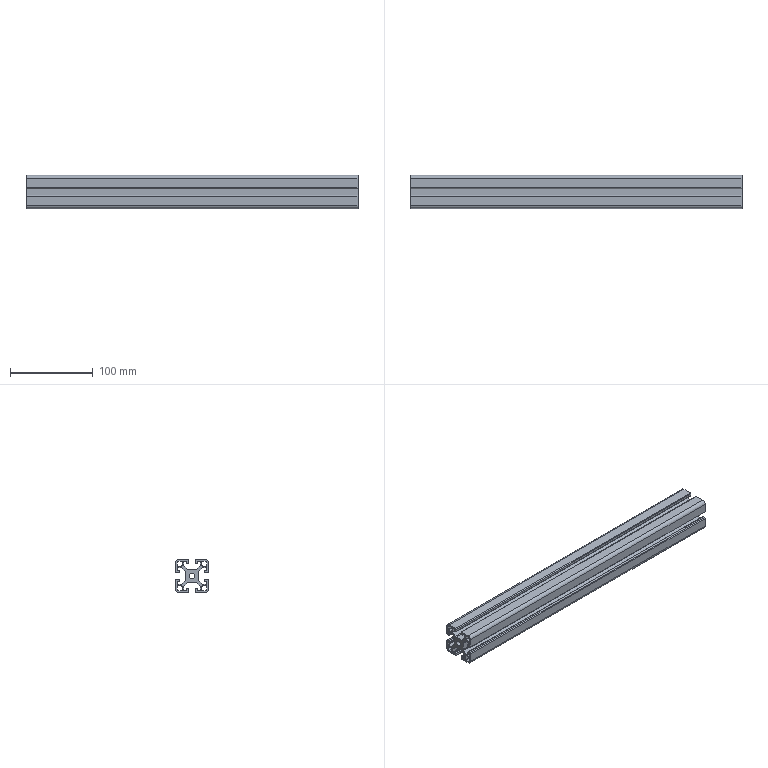Part | STEP file | 1 solid | 156 faces | box 400 x 40 x 40 mm | volume 268994 mm3 | cylinder 78 | plane 78 | commonest cylinder face diameters 1 x44 2 x16 4 x12 8 x4 6.5 x2